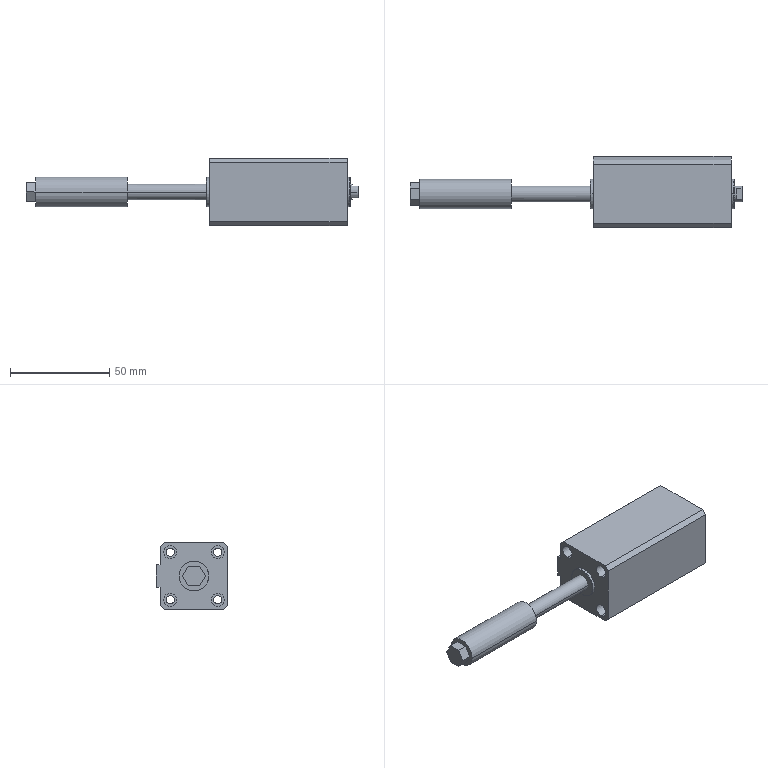Part | STEP file | Cylinder SDAJS 20×40-30 Retract | 2 solids | 90 faces | box 167.5 x 36 x 34 mm | volume 91234 mm3 | cylinder 40 | plane 38 | cone 8 | spline 4 | commonest cylinder face diameters 6.5 x16 4.2 x12 15 x6 3.3 x4 8 x2